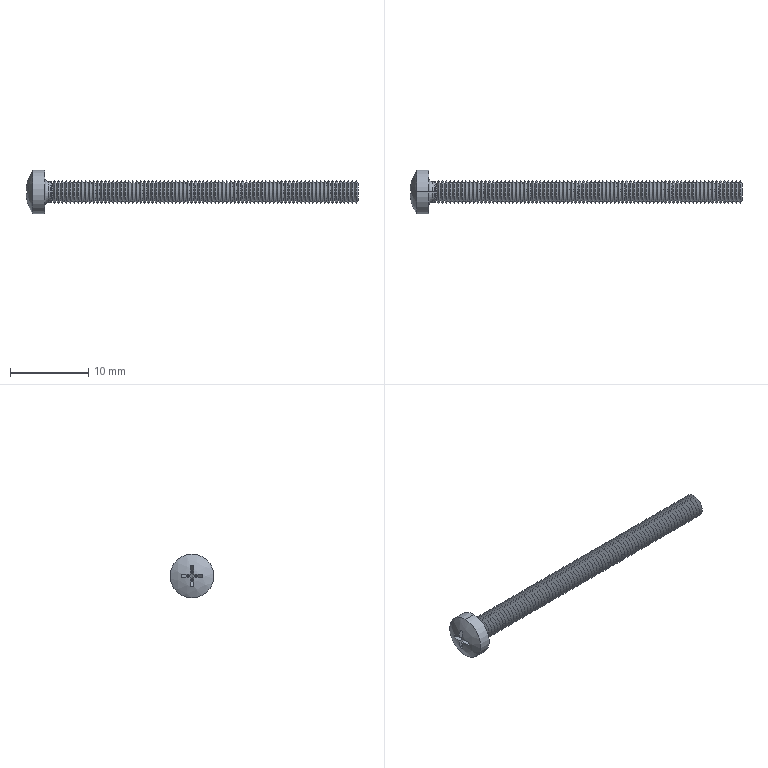Part | NX | features BREP 1 | 1 solid | 337 faces | box 42.388 x 5.6 x 5.6 mm | volume 256.849 mm3 | cone 316 | plane 14 | cylinder 4 | torus 2 | sphere 1 | commonest cylinder face diameters 2.598 x2 5.6 x2